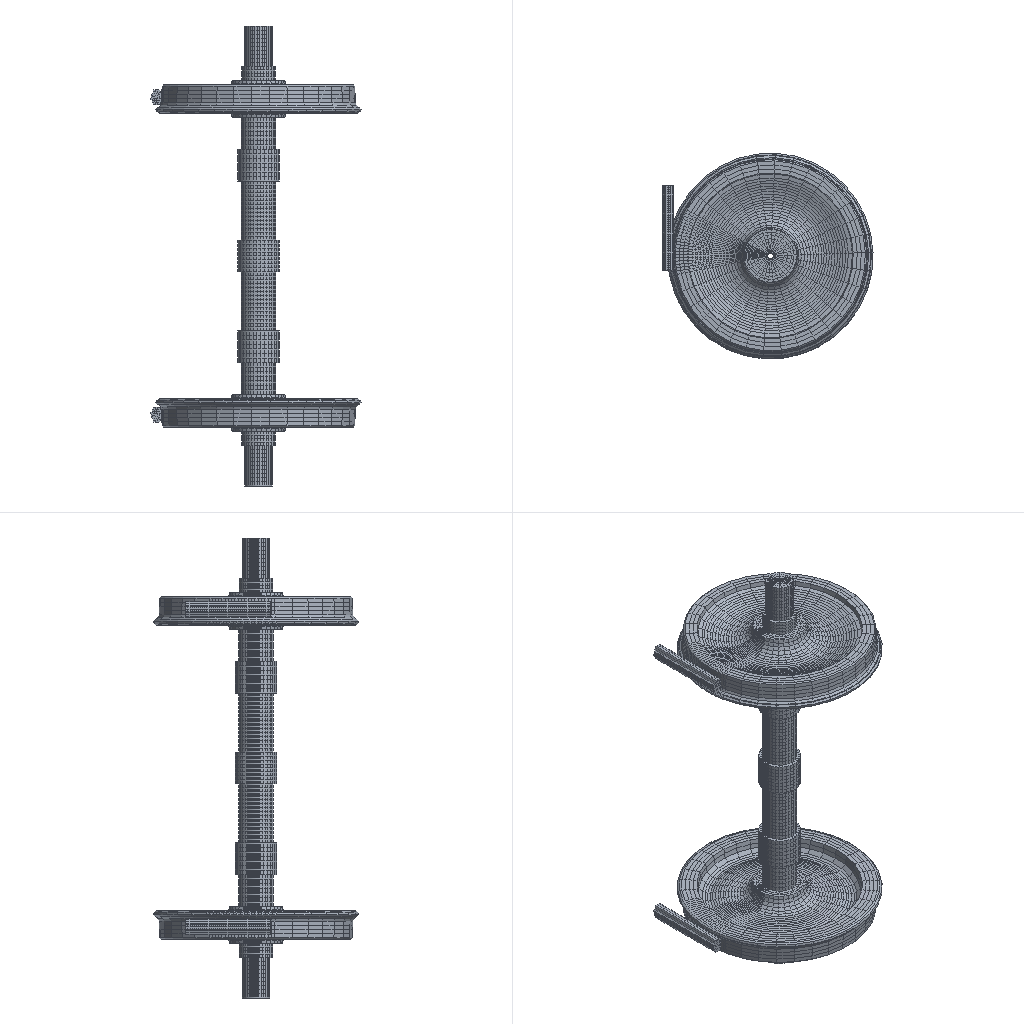Simulation study | abaqus
Set-up summary:
category,name,step,type,value,unit,region
solver,abaqus
solver,version,,,Abaqus/Standard 2020
units,not stated in the deck,,not stated
analysis,deck,,transient,transient
load_step,Step-1,Step-1,transient
load_step,Step-1-jingya,Step-1-jingya,transient
load_step,Step-2,Step-2,transient
load_step,requested,,,3
mesh,nodes,,,46650
mesh,elements,,,36840
element_type,C3D6,,solid,880
element_type,C3D8R,,solid,35960
load,load commands in deck,,count,3
bc,support commands in deck,,count,2
material,MATERIAL-RAIL,,in results
material,MATERIAL-WHEEL,,in results
check,setup vs results,,match,"per instance, exact: element labels, types and connectivity; labels of the nodes the elements use; coordinates of those nodes at SINGLE_PRECISION in 2 of 2 instance(s)"
Abaqus input file, long lists of numbers shortened:
*Heading
** Job name: Job-1 Model name: Model-1-step4-ur
** Generated by: Abaqus/CAE 2020
*Preprint, echo=NO, model=NO, history=NO, contact=NO
**
** PARTS
**
*Part, name=cu-rail
*Node
   6403,        1250.,   897.07,  -808.032
 219043,        1250.,         460.,  -828.032
** (3231 more lines like these left out)
*Element, type=C3D8R
9081052,3394664,3394672,3394670,3394665,3394675,3394676,3394677,3394678
9081053,3394675,3394676,3394677,3394678,3394679,3394680,3394681,3394682
** (2158 more lines like these left out)
*Element, type=C3D6
9081452,3394656,3394671,3394674,3394755,3395035,3394756
9081453,3394755,3395035,3394756,3394759,3395038,3394760
** (78 more lines like these left out)
*Elset, elset=_PickedSet2, internal
9081052,9081053,9081054,9081055,9081056,9081057,9081058,9081059,9081060,9081061,9081062,9081063,9081064,9081065,9081066,9081067
9081068,9081069,9081070,9081071,9081072,9081073,9081074,9081075,9081076,9081077,9081078,9081079,9081080,9081081,9081082,9081083
** (138 more lines like these left out)
** Section: Section-rail
*Solid Section, elset=_PickedSet2, material=Material-rail
,
*End Part
**
*Part, name=cu-wheel
*Node
   6403,        1250.,   897.07,  -808.032
   6419,   1127.402,   435.614,  -828.032
** (43415 more lines like these left out)
*Element, type=C3D8R
9083343,   6496,   6495,   6502,   6503,3397829,3397832,3397831,3397830
9083344,   6485,   6486,   6484,   6483,3397833,3397836,3397835,3397834
** (33798 more lines like these left out)
*Element, type=C3D6
9083367,   6463,   6470,   6462,3397868,3397864,3397870
9083372,   6464,   6456,   6457,3397869,3397874,3397876
** (798 more lines like these left out)
*Elset, elset=_PickedSet2, internal
9083343,9083344,9083345,9083346,9083347,9083348,9083349,9083350,9083351,9083352,9083353,9083354,9083355,9083356,9083357,9083358
9083359,9083360,9083361,9083362,9083363,9083364,9083365,9083366,9083367,9083368,9083369,9083370,9083371,9083372,9083373,9083374
** (2161 more lines like these left out)
** Section: Section-wheel
*Solid Section, elset=_PickedSet2, material=Material-wheel
,
*End Part
**
**
** ASSEMBLY
**
*Assembly, name=Assembly
**
*Instance, name=cu-rail-1, part=cu-rail
*End Instance
**
*Instance, name=cu-wheel-1, part=cu-wheel
*End Instance
**
*Node
      1,        1250.,         460.,           0.
*Node
      2,        1250.,         460.,  -991.032
*Nset, nset=Set-9
 1,
*Nset, nset=Set-10
 1,
*Nset, nset=Set-11
 1,
*Nset, nset=Set-L, instance=cu-wheel-1
3394604,
*Nset, nset=Set-LL, instance=cu-wheel-1
 788678, 788679, 788680, 788681, 788682, 788683, 788684, 788685, 788686, 788687, 788688,3398218,3398219,3398226,3398229,3398232
3398235,3398238,3398241,3398244,3398246,3398254,3398654,3398655,3398662,3398665,3398668,3398671,3398674,3398677,3398680,3398682
** (33 more lines like these left out)
*Nset, nset=Set-RAIL, instance=cu-rail-1
3394640,3394641,3394642,3395036,3395037,3395039,3395040,3395042,3395043,3395045,3395046,3395048,3395049,3395051,3395052,3395054
3395055,3395057,3395058,3395060,3395061,3395063,3395064,3395066,3395067,3395069,3395070,3395072,3395073,3395075,3395076,3395078
** (14 more lines like these left out)
*Nset, nset=Set-RR, instance=cu-wheel-1
3419790,3419791,3419792,3419793,3419794,3419795,3419796,3419797,3419798,3419799,3419800,3420075,3420083,3420085,3420088,3420091
3420094,3420097,3420100,3420103,3420110,3420111,3420511,3420519,3420521,3420524,3420527,3420530,3420533,3420536,3420539,3420546
** (33 more lines like these left out)
*Nset, nset=Set-left
 2,
*Nset, nset=Set-r, instance=cu-wheel-1
3394602,
*Nset, nset=Set-right
 1,
*Nset, nset=m_Set-8
 1,
*Elset, elset=_Surf-15_S3, internal, instance=cu-wheel-1
9094270,9094293,9094298,9094301,9094306,9094312,9094314,9094616,9094639,9094644,9094647,9094652,9094658,9094660,9094744,9094749
9094750,9094751,9094752,9094753,9094754,9094755,9094756,9094760,9094962,9094985,9094990,9094993,9094998,9095004,9095006,9095090
** (7 more lines like these left out)
*Elset, elset=_Surf-15_S4, internal, instance=cu-wheel-1
9094180,9094181,9094186,9094189,9094193,9094198,9094205,9094207,9094209,9094214,9094216,9094217,9094223,9094227,9094233,9094238
9094239,9094241,9094244,9094254,9094258,9094268,9094271,9094281,9094283,9094288,9094526,9094527,9094532,9094535,9094539,9094544
** (14 more lines like these left out)
*Elset, elset=_Surf-15_S5, internal, instance=cu-wheel-1
9111826,9111827,9111832,9111835,9111839,9111844,9111851,9111853,9111855,9111860,9111862,9111863,9111869,9111873,9111879,9111884
9111885,9111887,9111890,9111900,9111904,9111914,9111917,9111927,9111929,9111934,9112172,9112173,9112178,9112181,9112185,9112190
** (14 more lines like these left out)
*Elset, elset=_Surf-15_S6, internal, instance=cu-wheel-1
9111916,9111939,9111944,9111947,9111952,9111958,9111960,9112262,9112285,9112290,9112293,9112298,9112304,9112306,9112390,9112395
9112396,9112397,9112398,9112399,9112400,9112401,9112402,9112406,9112608,9112631,9112636,9112639,9112644,9112650,9112652,9112736
** (7 more lines like these left out)
*Surface, type=ELEMENT, name=Surf-15
_Surf-15_S3, S3
_Surf-15_S4, S4
_Surf-15_S6, S6
_Surf-15_S5, S5
*Elset, elset=_Surf-16_S3, internal, instance=cu-wheel-1, generate
9095207, 9096245,     346
*Elset, elset=_Surf-16_S4, internal, instance=cu-wheel-1
9095195,9095196,9095197,9095541,9095542,9095543,9095887,9095888,9095889,9096233,9096234,9096235
*Elset, elset=_Surf-16_S5, internal, instance=cu-wheel-1
9112841,9112842,9112843,9113187,9113188,9113189,9113533,9113534,9113535,9113879,9113880,9113881
*Elset, elset=_Surf-16_S6, internal, instance=cu-wheel-1, generate
9112853, 9113891,     346
*Surface, type=ELEMENT, name=Surf-16
_Surf-16_S3, S3
_Surf-16_S4, S4
_Surf-16_S6, S6
_Surf-16_S5, S5
*Elset, elset=_Surf-L_S4, internal, instance=cu-wheel-1
9083675,9084021,9084367,9084713,9085059,9085405,9085751,9086097,9086443,9086789,9087135,9087481,9087827,9088173,9088519,9088865
9089211,9089557,9089903,9090249,9090568,9090574,9090576,9090578,9090580,9090582,9090584,9090586,9090587,9090914,9090920,9090922
** (17 more lines like these left out)
*Elset, elset=_Surf-L_S5, internal, instance=cu-wheel-1
9083648,9083654,9083656,9083658,9083660,9083662,9083664,9083666,9083667,9083994,9084000,9084002,9084004,9084006,9084008,9084010
9084012,9084013,9084340,9084346,9084348,9084350,9084352,9084354,9084356,9084358,9084359,9084686,9084692,9084694,9084696,9084698
** (12 more lines like these left out)
*Surface, type=ELEMENT, name=Surf-L
_Surf-L_S4, S4
_Surf-L_S5, S5
*Elset, elset=_Surf-R_S4, internal, instance=cu-wheel-1
9101294,9101300,9101302,9101304,9101306,9101308,9101310,9101312,9101313,9101640,9101646,9101648,9101650,9101652,9101654,9101656
9101658,9101659,9101986,9101992,9101994,9101996,9101998,9102000,9102002,9102004,9102005,9102332,9102338,9102340,9102342,9102344
** (12 more lines like these left out)
*Elset, elset=_Surf-R_S5, internal, instance=cu-wheel-1
9101321,9101667,9102013,9102359,9102705,9103051,9103397,9103743,9104089,9104435,9104781,9105127,9105473,9105819,9106165,9106511
9106857,9107203,9107549,9107895,9108214,9108220,9108222,9108224,9108226,9108228,9108230,9108232,9108233,9108560,9108566,9108568
** (17 more lines like these left out)
*Surface, type=ELEMENT, name=Surf-R
_Surf-R_S4, S4
_Surf-R_S5, S5
*Elset, elset=_Surf-ll_S3, internal, instance=cu-wheel-1
9083451,9083458,9083459,9083465,9083473,9083477,9083478,9083484,9083487,9083493,9083496,9083502,9083504,9083508,9083511,9083517
9083521,9083525,9083529,9083531,9083536,9083540,9083550,9083551,9083554,9083565,9083600,9083601,9083605,9083611,9083614,9083616
** (45 more lines like these left out)
*Elset, elset=_Surf-ll_S4, internal, instance=cu-wheel-1
9083548,9083573,9083578,9083585,9083590,9083591,9083593,9083675,9083894,9083919,9083924,9083931,9083936,9083937,9083939,9084021
9084240,9084265,9084270,9084277,9084282,9084283,9084285,9084367,9084586,9084611,9084616,9084623,9084628,9084629,9084631,9084713
** (31 more lines like these left out)
*Elset, elset=_Surf-ll_S5, internal, instance=cu-wheel-1
9083645,9083648,9083651,9083654,9083656,9083658,9083660,9083662,9083664,9083666,9083667,9083685,9083991,9083994,9083997,9084000
9084002,9084004,9084006,9084008,9084010,9084012,9084013,9084031,9084337,9084340,9084343,9084346,9084348,9084350,9084352,9084354
** (28 more lines like these left out)
*Elset, elset=_Surf-ll_S6, internal, instance=cu-wheel-1
9083676,9084022,9084368,9084714,9085060,9085406,9085752,9086098,9086444,9086790,9087136,9087482,9087828,9088174,9088520,9088866
9089212,9089558,9089904,9090250,9090371,9090378,9090379,9090385,9090393,9090397,9090398,9090404,9090407,9090413,9090416,9090422
** (67 more lines like these left out)
*Surface, type=ELEMENT, name=Surf-ll
_Surf-ll_S3, S3
_Surf-ll_S4, S4
_Surf-ll_S6, S6
_Surf-ll_S5, S5
*Elset, elset=_Surf-rail_S4, internal, instance=cu-rail-1
9081663,9081664,9081665,9081666,9081667,9081668,9081669,9081670,9081671,9081672,9081673,9081774,9081775,9081776,9081777,9081778
9081779,9081780,9081781,9081782,9081783,9081784,9081785,9081786,9081787,9081788,9081789,9081790,9081791,9081792,9081793,9081994
** (16 more lines like these left out)
*Elset, elset=_Surf-rail_S5, internal, instance=cu-rail-1
9081092,9081093,9081094,9081095,9081096,9081097,9081098,9081099,9081100,9081101,9081102,9081103,9081104,9081105,9081106,9081107
9081108,9081109,9081110,9081111,9081152,9081153,9081154,9081155,9081156,9081157,9081158,9081159,9081160,9081161,9081162,9081163
** (16 more lines like these left out)
*Surface, type=ELEMENT, name=Surf-rail
_Surf-rail_S4, S4
_Surf-rail_S5, S5
*Elset, elset=_Surf-rr_S3, internal, instance=cu-wheel-1
9101322,9101668,9102014,9102360,9102706,9103052,9103398,9103744,9104090,9104436,9104782,9105128,9105474,9105820,9106166,9106512
9106858,9107204,9107550,9107896,9108017,9108024,9108025,9108031,9108039,9108043,9108044,9108050,9108053,9108059,9108062,9108068
** (67 more lines like these left out)
*Elset, elset=_Surf-rr_S4, internal, instance=cu-wheel-1
9101291,9101294,9101297,9101300,9101302,9101304,9101306,9101308,9101310,9101312,9101313,9101331,9101637,9101640,9101643,9101646
9101648,9101650,9101652,9101654,9101656,9101658,9101659,9101677,9101983,9101986,9101989,9101992,9101994,9101996,9101998,9102000
** (28 more lines like these left out)
*Elset, elset=_Surf-rr_S5, internal, instance=cu-wheel-1
9101194,9101219,9101224,9101231,9101236,9101237,9101239,9101321,9101540,9101565,9101570,9101577,9101582,9101583,9101585,9101667
9101886,9101911,9101916,9101923,9101928,9101929,9101931,9102013,9102232,9102257,9102262,9102269,9102274,9102275,9102277,9102359
** (31 more lines like these left out)
*Elset, elset=_Surf-rr_S6, internal, instance=cu-wheel-1
9101097,9101104,9101105,9101111,9101119,9101123,9101124,9101130,9101133,9101139,9101142,9101148,9101150,9101154,9101157,9101163
9101167,9101171,9101175,9101177,9101182,9101186,9101196,9101197,9101200,9101211,9101246,9101247,9101251,9101257,9101260,9101262
** (45 more lines like these left out)
*Surface, type=ELEMENT, name=Surf-rr
_Surf-rr_S3, S3
_Surf-rr_S4, S4
_Surf-rr_S6, S6
_Surf-rr_S5, S5
*Elset, elset=_Surf-wheel_S3, internal, instance=cu-wheel-1
9090363,9090709,9091055,9091401,9091747,9092093,9092439,9092785,9093131,9093477,9093823,9094169,9094515,9094861,9095207,9095553
9095899,9096245,9096591,9096937,9097283,9097629,9097975,9098321,9098667,9099013,9099359,9099705,9100051,9100397,9101089,9101435
** (2 more lines like these left out)
*Elset, elset=_Surf-wheel_S4, internal, instance=cu-wheel-1
9090351,9090352,9090353,9090354,9090357,9090697,9090698,9090699,9090700,9090703,9091043,9091044,9091045,9091046,9091049,9091389
9091390,9091391,9091392,9091395,9091735,9091736,9091737,9091738,9091741,9092081,9092082,9092083,9092084,9092087,9092427,9092428
** (14 more lines like these left out)
*Elset, elset=_Surf-wheel_S5, internal, instance=cu-wheel-1
9083431,9083432,9083433,9083434,9083437,9083777,9083778,9083779,9083780,9083783,9084123,9084124,9084125,9084126,9084129,9084469
9084470,9084471,9084472,9084475,9084815,9084816,9084817,9084818,9084821,9085161,9085162,9085163,9085164,9085167,9085507,9085508
** (14 more lines like these left out)
*Elset, elset=_Surf-wheel_S6, internal, instance=cu-wheel-1
9083443,9083789,9084135,9084481,9084827,9085173,9085519,9085865,9086211,9086557,9086903,9087249,9087595,9087941,9088287,9088633
9088979,9089325,9089671,9090017,9108009,9108355,9108701,9109047,9109393,9109739,9110085,9110431,9110777,9111123,9111469,9111815
** (2 more lines like these left out)
*Surface, type=ELEMENT, name=Surf-wheel
_Surf-wheel_S3, S3
_Surf-wheel_S4, S4
_Surf-wheel_S6, S6
_Surf-wheel_S5, S5
*Elset, elset=_m_Surf-8_S3, internal, instance=cu-wheel-1
9101089,9101095,9101435,9101441,9101781,9101787,9102127,9102133,9102473,9102479,9102819,9102825,9103165,9103171,9103511,9103517
9103857,9103863,9104203,9104209,9104549,9104555,9104895,9104901,9105241,9105247,9105587,9105593,9105933,9105939,9106279,9106285
** (3 more lines like these left out)
*Elset, elset=_m_Surf-8_S4, internal, instance=cu-wheel-1
9101077,9101078,9101079,9101080,9101083,9101094,9101423,9101424,9101425,9101426,9101429,9101440,9101769,9101770,9101771,9101772
9101775,9101786,9102115,9102116,9102117,9102118,9102121,9102132,9102461,9102462,9102463,9102464,9102467,9102478,9102807,9102808
** (6 more lines like these left out)
*Elset, elset=_m_Surf-8_S5, internal, instance=cu-wheel-1
9107997,9107998,9107999,9108000,9108003,9108014,9108343,9108344,9108345,9108346,9108349,9108360,9108689,9108690,9108691,9108692
9108695,9108706,9109035,9109036,9109037,9109038,9109041,9109052,9109381,9109382,9109383,9109384,9109387,9109398,9109727,9109728
** (10 more lines like these left out)
*Elset, elset=_m_Surf-8_S6, internal, instance=cu-wheel-1
9101095,9101441,9101787,9102133,9102479,9102825,9103171,9103517,9103863,9104209,9104555,9104901,9105247,9105593,9105939,9106285
9106631,9106977,9107323,9107669,9108009,9108015,9108355,9108361,9108701,9108707,9109047,9109053,9109393,9109399,9109739,9109745
** (3 more lines like these left out)
*Surface, type=ELEMENT, name=m_Surf-8
_m_Surf-8_S3, S3
_m_Surf-8_S4, S4
_m_Surf-8_S6, S6
_m_Surf-8_S5, S5
*Elset, elset=_m_Surf-10_S3, internal, instance=cu-wheel-1
9090363,9090369,9090709,9090715,9091055,9091061,9091401,9091407,9091747,9091753,9092093,9092099,9092439,9092445,9092785,9092791
9093131,9093137,9093477,9093483,9093823,9093829,9094169,9094175,9094515,9094521,9094861,9094867,9095207,9095213,9095553,9095559
** (2 more lines like these left out)
*Elset, elset=_m_Surf-10_S4, internal, instance=cu-wheel-1
9090351,9090352,9090353,9090354,9090357,9090368,9090697,9090698,9090699,9090700,9090703,9090714,9091043,9091044,9091045,9091046
9091049,9091060,9091389,9091390,9091391,9091392,9091395,9091406,9091735,9091736,9091737,9091738,9091741,9091752,9092081,9092082
** (10 more lines like these left out)
*Elset, elset=_m_Surf-10_S5, internal, instance=cu-wheel-1
9083431,9083432,9083433,9083434,9083437,9083448,9083777,9083778,9083779,9083780,9083783,9083794,9084123,9084124,9084125,9084126
9084129,9084140,9084469,9084470,9084471,9084472,9084475,9084486,9084815,9084816,9084817,9084818,9084821,9084832,9085161,9085162
** (6 more lines like these left out)
*Elset, elset=_m_Surf-10_S6, internal, instance=cu-wheel-1
9083443,9083449,9083789,9083795,9084135,9084141,9084481,9084487,9084827,9084833,9085173,9085179,9085519,9085525,9085865,9085871
9086211,9086217,9086557,9086563,9086903,9086909,9087249,9087255,9087595,9087601,9087941,9087947,9088287,9088293,9088633,9088639
** (1 more lines like these left out)
*Surface, type=ELEMENT, name=m_Surf-10
_m_Surf-10_S3, S3
_m_Surf-10_S4, S4
_m_Surf-10_S6, S6
_m_Surf-10_S5, S5
*Elset, elset=_s_Surf-7_S3, internal, instance=cu-wheel-1
9083451,9083458,9083459,9083465,9083473,9083478,9083484,9083487,9083493,9083496,9083502,9083504,9083508,9083511,9083517,9083521
9083525,9083529,9083531,9083797,9083804,9083805,9083811,9083819,9083824,9083830,9083833,9083839,9083842,9083848,9083850,9083854
** (58 more lines like these left out)
*Elset, elset=_s_Surf-7_S4, internal, instance=cu-wheel-1
9083454,9083800,9084146,9084492,9084838,9085184,9085530,9085876,9086222,9086568,9086914,9087260,9087606,9087952,9088298,9088644
9088990,9089336,9089682,9090028,9090374,9090375,9090380,9090383,9090387,9090392,9090399,9090403,9090408,9090410,9090411,9090417
** (61 more lines like these left out)
*Elset, elset=_s_Surf-7_S5, internal, instance=cu-wheel-1
9083454,9083455,9083460,9083463,9083467,9083472,9083479,9083483,9083488,9083490,9083491,9083497,9083501,9083507,9083512,9083513
9083515,9083518,9083528,9083800,9083801,9083806,9083809,9083813,9083818,9083825,9083829,9083834,9083836,9083837,9083843,9083847
** (61 more lines like these left out)
*Elset, elset=_s_Surf-7_S6, internal, instance=cu-wheel-1
9090371,9090378,9090379,9090385,9090393,9090398,9090404,9090407,9090413,9090416,9090422,9090424,9090428,9090431,9090437,9090441
9090445,9090449,9090451,9090717,9090724,9090725,9090731,9090739,9090744,9090750,9090753,9090759,9090762,9090768,9090770,9090774
** (58 more lines like these left out)
*Surface, type=ELEMENT, name=s_Surf-7
_s_Surf-7_S3, S3
_s_Surf-7_S4, S4
_s_Surf-7_S6, S6
_s_Surf-7_S5, S5
*Elset, elset=_s_Surf-8_S4, internal, instance=cu-rail-1
9082223,9082224,9082225,9082226,9082227,9082228,9082229,9082230,9082231,9082232,9082233,9082894,9082895,9082896,9082897,9082898
9082899,9082900,9082901,9082902,9082903,9082904,9082905,9082906,9082907,9082908,9082909,9082910,9082911,9082912,9082913,9083114
** (5 more lines like these left out)
*Elset, elset=_s_Surf-8_S5, internal, instance=cu-rail-1
9082274,9082275,9082276,9082277,9082278,9082279,9082280,9082281,9082282,9082403,9082404,9082405,9082406,9082407,9082408,9082409
9082410,9082411,9082412,9082413,9082414,9082415,9082416,9082417,9082418,9082419,9082420,9082421,9082422,9082423,9082424,9082425
** (5 more lines like these left out)
*Surface, type=ELEMENT, name=s_Surf-8
_s_Surf-8_S4, S4
_s_Surf-8_S5, S5
*Elset, elset=_s_Surf-10_S4, internal, instance=cu-rail-1
9081663,9081664,9081665,9081666,9081667,9081668,9081669,9081670,9081671,9081672,9081673,9081774,9081775,9081776,9081777,9081778
9081779,9081780,9081781,9081782,9081783,9081784,9081785,9081786,9081787,9081788,9081789,9081790,9081791,9081792,9081793,9081994
** (5 more lines like these left out)
*Elset, elset=_s_Surf-10_S5, internal, instance=cu-rail-1
9081092,9081093,9081094,9081095,9081096,9081097,9081098,9081099,9081100,9081101,9081102,9081103,9081104,9081105,9081106,9081107
9081108,9081109,9081110,9081111,9081232,9081233,9081234,9081235,9081236,9081237,9081238,9081239,9081240,9081241,9081242,9081243
** (5 more lines like these left out)
*Surface, type=ELEMENT, name=s_Surf-10
_s_Surf-10_S4, S4
_s_Surf-10_S5, S5
*Elset, elset=_s_Surf-12_S3, internal, instance=cu-wheel-1
9090592,9090597,9090598,9090599,9090600,9090601,9090602,9090603,9090604,9090608,9090938,9090943,9090944,9090945,9090946,9090947
9090948,9090949,9090950,9090954,9091284,9091289,9091290,9091291,9091292,9091293,9091294,9091295,9091296,9091300,9091630,9091635
** (30 more lines like these left out)
*Elset, elset=_s_Surf-12_S4, internal, instance=cu-wheel-1
9083675,9084021,9084367,9084713,9085059,9085405,9085751,9086097,9086443,9086789,9087135,9087481,9087827,9088173,9088519,9088865
9089211,9089557,9089903,9090249,9090566,9090568,9090574,9090576,9090578,9090580,9090582,9090584,9090586,9090587,9090595,9090608
** (39 more lines like these left out)
*Elset, elset=_s_Surf-12_S5, internal, instance=cu-wheel-1
9083646,9083648,9083654,9083656,9083658,9083660,9083662,9083664,9083666,9083667,9083675,9083688,9083992,9083994,9084000,9084002
9084004,9084006,9084008,9084010,9084012,9084013,9084021,9084034,9084338,9084340,9084346,9084348,9084350,9084352,9084354,9084356
** (39 more lines like these left out)
*Elset, elset=_s_Surf-12_S6, internal, instance=cu-wheel-1
9083672,9083677,9083678,9083679,9083680,9083681,9083682,9083683,9083684,9083688,9084018,9084023,9084024,9084025,9084026,9084027
9084028,9084029,9084030,9084034,9084364,9084369,9084370,9084371,9084372,9084373,9084374,9084375,9084376,9084380,9084710,9084715
** (30 more lines like these left out)
*Surface, type=ELEMENT, name=s_Surf-12
_s_Surf-12_S3, S3
_s_Surf-12_S4, S4
_s_Surf-12_S6, S6
_s_Surf-12_S5, S5
*Elset, elset=_s_Surf-13_S3, internal, instance=cu-wheel-1
9083451,9083458,9083459,9083465,9083797,9083804,9083805,9083811,9084143,9084150,9084151,9084157,9084489,9084496,9084497,9084503
9084835,9084842,9084843,9084849,9085181,9085188,9085189,9085195,9085527,9085534,9085535,9085541,9085873,9085880,9085881,9085887
** (11 more lines like these left out)
*Elset, elset=_s_Surf-13_S4, internal, instance=cu-wheel-1
9090374,9090375,9090383,9090387,9090720,9090721,9090729,9090733,9091066,9091067,9091075,9091079,9091412,9091413,9091421,9091425
9091758,9091759,9091767,9091771,9092104,9092105,9092113,9092117,9092450,9092451,9092459,9092463,9092796,9092797,9092805,9092809
** (11 more lines like these left out)
*Elset, elset=_s_Surf-13_S5, internal, instance=cu-wheel-1
9083454,9083455,9083463,9083467,9083800,9083801,9083809,9083813,9084146,9084147,9084155,9084159,9084492,9084493,9084501,9084505
9084838,9084839,9084847,9084851,9085184,9085185,9085193,9085197,9085530,9085531,9085539,9085543,9085876,9085877,9085885,9085889
** (11 more lines like these left out)
*Elset, elset=_s_Surf-13_S6, internal, instance=cu-wheel-1
9090371,9090378,9090379,9090385,9090717,9090724,9090725,9090731,9091063,9091070,9091071,9091077,9091409,9091416,9091417,9091423
9091755,9091762,9091763,9091769,9092101,9092108,9092109,9092115,9092447,9092454,9092455,9092461,9092793,9092800,9092801,9092807
** (11 more lines like these left out)
*Surface, type=ELEMENT, name=s_Surf-13
_s_Surf-13_S3, S3
_s_Surf-13_S4, S4
_s_Surf-13_S6, S6
_s_Surf-13_S5, S5
*Elset, elset=_s_Surf-14_S3, internal, instance=cu-wheel-1
9083451,9083458,9083459,9083465,9083473,9083477,9083478,9083484,9083487,9083493,9083496,9083502,9083504,9083508,9083511,9083517
9083521,9083525,9083529,9083531,9083536,9083540,9083550,9083551,9083554,9083565,9083797,9083804,9083805,9083811,9083819,9083823
** (105 more lines like these left out)
*Elset, elset=_s_Surf-14_S4, internal, instance=cu-wheel-1
9083454,9083542,9083548,9083573,9083578,9083585,9083590,9083591,9083593,9083800,9083888,9083894,9083919,9083924,9083931,9083936
9083937,9083939,9084146,9084234,9084240,9084265,9084270,9084277,9084282,9084283,9084285,9084492,9084580,9084586,9084611,9084616
** (108 more lines like these left out)
*Elset, elset=_s_Surf-14_S5, internal, instance=cu-wheel-1
9083454,9083455,9083460,9083463,9083467,9083472,9083479,9083481,9083483,9083488,9083490,9083491,9083497,9083501,9083507,9083512
9083513,9083515,9083518,9083528,9083532,9083542,9083545,9083555,9083557,9083562,9083800,9083801,9083806,9083809,9083813,9083818
** (108 more lines like these left out)
*Elset, elset=_s_Surf-14_S6, internal, instance=cu-wheel-1
9083544,9083557,9083567,9083572,9083575,9083580,9083586,9083588,9083890,9083903,9083913,9083918,9083921,9083926,9083932,9083934
9084236,9084249,9084259,9084264,9084267,9084272,9084278,9084280,9084582,9084595,9084605,9084610,9084613,9084618,9084624,9084626
** (105 more lines like these left out)
*Surface, type=ELEMENT, name=s_Surf-14
_s_Surf-14_S3, S3
_s_Surf-14_S4, S4
_s_Surf-14_S6, S6
_s_Surf-14_S5, S5
** Constraint: Constraint-1
*Coupling, constraint name=Constraint-1, ref node=m_Set-8, surface=s_Surf-14
*Kinematic
*End Assembly
*Amplitude, name=Amp-1
             0.,              0.,          0.0013,              1.
*Amplitude, name=Amp-3
             0.,              0.,              1.,              1.
*Amplitude, name=gravity, definition=SMOOTH STEP
             0.,              0.,          0.0013,              1.,            0.01,              1.
**
** MATERIALS
**
*Material, name=Material-rail
*Density
 7.8e-09,
*Elastic
210000., 0.29
*Material, name=Material-wheel
*Density
 7.85e-09,
*Elastic
210000., 0.3
**
** INTERACTION PROPERTIES
**
*Surface Interaction, name=IntProp-1
1.,
*Friction, slip tolerance=0.005
 0.3,
*Surface Behavior, pressure-overclosure=HARD
**
** BOUNDARY CONDITIONS
**
** Name: [REDACTED] : Symmetric / antisymmetric / fully fixed
*Boundary
Set-RAIL, ENCASTRE
**
** INTERACTIONS
**
** Interaction: Int-2
*Contact
*Contact Inclusions, ALL EXTERIOR
*Contact Property Assignment
 ,  , IntProp-1
** Interaction: Int-3
*Contact Pair, interaction=IntProp-1, type=SURFACE TO SURFACE
s_Surf-8, m_Surf-8
** Interaction: Int-4
*Contact Pair, interaction=IntProp-1, type=SURFACE TO SURFACE
s_Surf-10, m_Surf-10
** ----------------------------------------------------------------
**
** STEP: Step-1
**
*Step, name=Step-1, nlgeom=YES, inc=1000
*Dynamic
0.01,1.,1e-05
**
** LOADS
**
** Name: Load-2   Type: Gravity
*Dload
, GRAV, 9800., -1., 0., 0.
**
** CONTROLS
**
*Controls, reset
*Controls, parameters=time incrementation
, , , , , , , 20, , ,
**
** OUTPUT REQUESTS
**
*Restart, write, frequency=0
**
** FIELD OUTPUT: F-Output-1
**
*Output, field, frequency=1
*Node Output
CF, RF, U, V
*Element Output, directions=YES
E, LE, MISES, PE, PEEQ, PEMAG, S
*Contact Output
CDISP, CSTRESS
**
** HISTORY OUTPUT: H-Output-1
**
*Output, history, frequency=1
*Contact Output, master=m_Surf-8, slave=s_Surf-8
CAREA, CDISP, CFN1, CFN2, CFN3, CFNM, CFS1, CFS2, CFS3, CFSM, CFT1, CFT2, CFT3, CFTM, CMN1, CMN2
CMN3, CMNM, CMS1, CMS2, CMS3, CMSM, CMT1, CMT2, CMT3, CMTM, CSTRESS, CTRQ
*End Step
** ----------------------------------------------------------------
**
** STEP: Step-1-jingya
**
*Step, name=Step-1-jingya, nlgeom=YES, inc=1000
*Dynamic
0.01,1.,1e-05
**
** LOADS
**
** Name: Load-1   Type: Concentrated force
*Cload, amplitude=Amp-3
Set-10, 1, -125000.
**
** OUTPUT REQUESTS
**
*Restart, write, frequency=0
**
** FIELD OUTPUT: F-Output-1
**
*Output, field, frequency=1
*Node Output
CF, RF, U, V
*Element Output, directions=YES
E, LE, MISES, PE, PEEQ, PEMAG, S
*Contact Output
CDISP, CSTRESS
**
** HISTORY OUTPUT: H-Output-1
**
*Output, history, frequency=1
*Contact Output, master=m_Surf-8, slave=s_Surf-8
CAREA, CDISP, CFN1, CFN2, CFN3, CFNM, CFS1, CFS2, CFS3, CFSM, CFT1, CFT2, CFT3, CFTM, CMN1, CMN2
CMN3, CMNM, CMS1, CMS2, CMS3, CMSM, CMT1, CMT2, CMT3, CMTM, CSTRESS, CTRQ
*End Step
** ----------------------------------------------------------------
**
** STEP: Step-2
**
*Step, name=Step-2, nlgeom=YES, inc=1000
*Dynamic
1.,1.,1e-05
**
** BOUNDARY CONDITIONS
**
** Name: BC-2 Type: 位移/转角
*Boundary
Set-11, 6, 6, 0.26
**
** LOADS
**
** Name: Load-1   Type: Concentrated force
*Cload
**
** OUTPUT REQUESTS
**
*Restart, write, frequency=0
**
** FIELD OUTPUT: F-Output-1
**
*Output, field, frequency=1
*Node Output
A, CF, RF, U, V
*Element Output, directions=YES
E, LE, MISES, PE, PEEQ, PEMAG, S
*Contact Output
CDISP, CSTRESS
**
** FIELD OUTPUT: F-Output-2
**
*Node Output
CF, RF, U, V
*Element Output, directions=YES
E, LE, MISES, PE, PEEQ, PEMAG, S
*Contact Output
CDISP, CSTRESS
**
** HISTORY OUTPUT: H-Output-1
**
*Output, history, frequency=1
*Contact Output, master=m_Surf-8, slave=s_Surf-8
CAREA, CDISP, CFN1, CFN2, CFN3, CFNM, CFS1, CFS2, CFS3, CFSM, CFT1, CFT2, CFT3, CFTM, CMN1, CMN2
CMN3, CMNM, CMS1, CMS2, CMS3, CMSM, CMT1, CMT2, CMT3, CMTM, CSTRESS, CTRQ
**
** HISTORY OUTPUT: H-Output-2
**
*Contact Output, master=m_Surf-10, slave=s_Surf-10
CAREA, CDISP, CFN1, CFN2, CFN3, CFNM, CFS1, CFS2, CFS3, CFSM, CFT1, CFT2, CFT3, CFTM, CMN1, CMN2
CMN3, CMNM, CMS1, CMS2, CMS3, CMSM, CMT1, CMT2, CMT3, CMTM, CSTRESS, CTRQ
*End Step
Results summary:
result,step,,completed,increments=23 time=1.0/1.0
result,step,,completed,increments=17 time=1.0/1.0
result,step,,completed,increments=12 time=1.0/1.0
result,analysis,,,transient
result,last_loadstep,,,3
result,primary field,,,U
result,reaction total,,FX,135869.181,model units
result,reaction total,,FY,5.162,model units
result,reaction total,,FZ,-0.02646,model units